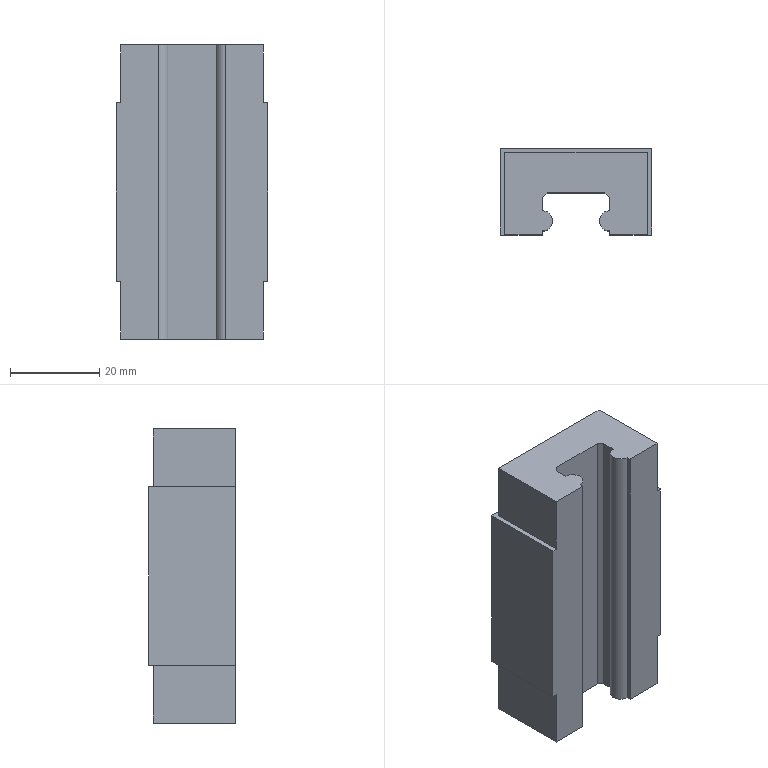Part | Creo | features CURVE 3, DATUM PLANE 3, PROTRUSION 2, COORDINATE SYSTEM 1, CUT 1 | 1 solid | 36 faces | box 34 x 19.4 x 66 mm | volume 33141 mm3 | plane 26 | cylinder 10 | commonest cylinder face diameters 3.3 x8 4.48 x2
STEP:
#1=CARTESIAN_POINT('',(0.,0.,0.));
#2=DIRECTION('',(0.,0.,1.));
#3=DIRECTION('',(1.,0.,0.));
#4=AXIS2_PLACEMENT_3D('',#1,#2,#3);
#5=CARTESIAN_POINT('',(16.,18.4,-20.));
#6=VERTEX_POINT('',#5);
#7=CARTESIAN_POINT('',(-16.,18.4,-20.));
#8=VERTEX_POINT('',#7);
#9=CARTESIAN_POINT('',(16.,18.4,-20.));
#10=DIRECTION('',(-1.,0.,0.));
#11=VECTOR('',#10,32.);
#12=LINE('',#9,#11);
#13=EDGE_CURVE('',#6,#8,#12,.T.);
#14=ORIENTED_EDGE('',*,*,#13,.F.);
#15=CARTESIAN_POINT('',(16.,0.,-20.));
#16=VERTEX_POINT('',#15);
#17=CARTESIAN_POINT('',(16.,0.,-20.));
#18=DIRECTION('',(0.,1.,0.));
#19=VECTOR('',#18,18.4);
#20=LINE('',#17,#19);
#21=EDGE_CURVE('',#16,#6,#20,.T.);
#22=ORIENTED_EDGE('',*,*,#21,.F.);
#23=CARTESIAN_POINT('',(17.,0.,-20.));
#24=VERTEX_POINT('',#23);
#25=CARTESIAN_POINT('',(16.,0.,-20.));
#26=DIRECTION('',(1.,0.,0.));
#27=VECTOR('',#26,1.);
#28=LINE('',#25,#27);
#29=EDGE_CURVE('',#16,#24,#28,.T.);
#30=ORIENTED_EDGE('',*,*,#29,.T.);
#31=CARTESIAN_POINT('',(17.,19.4,-20.));
#32=VERTEX_POINT('',#31);
#33=CARTESIAN_POINT('',(17.,0.,-20.));
#34=DIRECTION('',(0.,1.,0.));
#35=VECTOR('',#34,19.4);
#36=LINE('',#33,#35);
#37=EDGE_CURVE('',#24,#32,#36,.T.);
#38=ORIENTED_EDGE('',*,*,#37,.T.);
#39=CARTESIAN_POINT('',(-17.,19.4,-20.));
#40=VERTEX_POINT('',#39);
#41=CARTESIAN_POINT('',(17.,19.4,-20.));
#42=DIRECTION('',(-1.,0.,0.));
#43=VECTOR('',#42,34.);
#44=LINE('',#41,#43);
#45=EDGE_CURVE('',#32,#40,#44,.T.);
#46=ORIENTED_EDGE('',*,*,#45,.T.);
#47=CARTESIAN_POINT('',(-17.,0.,-20.));
#48=VERTEX_POINT('',#47);
#49=CARTESIAN_POINT('',(-17.,19.4,-20.));
#50=DIRECTION('',(0.,-1.,0.));
#51=VECTOR('',#50,19.4);
#52=LINE('',#49,#51);
#53=EDGE_CURVE('',#40,#48,#52,.T.);
#54=ORIENTED_EDGE('',*,*,#53,.T.);
#55=CARTESIAN_POINT('',(-16.,0.,-20.));
#56=VERTEX_POINT('',#55);
#57=CARTESIAN_POINT('',(-17.,0.,-20.));
#58=DIRECTION('',(1.,0.,0.));
#59=VECTOR('',#58,1.);
#60=LINE('',#57,#59);
#61=EDGE_CURVE('',#48,#56,#60,.T.);
#62=ORIENTED_EDGE('',*,*,#61,.T.);
#63=CARTESIAN_POINT('',(-16.,0.,-20.));
#64=DIRECTION('',(0.,1.,0.));
#65=VECTOR('',#64,18.4);
#66=LINE('',#63,#65);
#67=EDGE_CURVE('',#56,#8,#66,.T.);
#68=ORIENTED_EDGE('',*,*,#67,.T.);
#69=EDGE_LOOP('',(#14,#22,#30,#38,#46,#54,#62,#68));
#70=FACE_OUTER_BOUND('',#69,.F.);
#71=CARTESIAN_POINT('',(0.,0.,-20.));
#72=DIRECTION('',(0.,0.,1.));
#73=DIRECTION('',(1.,0.,0.));
#74=AXIS2_PLACEMENT_3D('',#71,#72,#73);
#75=PLANE('',#74);
#76=ADVANCED_FACE('',(#70),#75,.F.);
#77=ORIENTED_EDGE('',*,*,#13,.T.);
#78=CARTESIAN_POINT('',(-16.,18.4,-33.));
#79=VERTEX_POINT('',#78);
#80=CARTESIAN_POINT('',(-16.,18.4,-33.));
#81=DIRECTION('',(0.,0.,1.));
#82=VECTOR('',#81,13.);
#83=LINE('',#80,#82);
#84=EDGE_CURVE('',#79,#8,#83,.T.);
#85=ORIENTED_EDGE('',*,*,#84,.F.);
#86=CARTESIAN_POINT('',(16.,18.4,-33.));
#87=VERTEX_POINT('',#86);
#88=CARTESIAN_POINT('',(16.,18.4,-33.));
#89=DIRECTION('',(-1.,0.,0.));
#90=VECTOR('',#89,32.);
#91=LINE('',#88,#90);
#92=EDGE_CURVE('',#87,#79,#91,.T.);
#93=ORIENTED_EDGE('',*,*,#92,.F.);
#94=CARTESIAN_POINT('',(16.,18.4,-33.));
#95=DIRECTION('',(0.,0.,1.));
#96=VECTOR('',#95,13.);
#97=LINE('',#94,#96);
#98=EDGE_CURVE('',#87,#6,#97,.T.);
#99=ORIENTED_EDGE('',*,*,#98,.T.);
#100=EDGE_LOOP('',(#77,#85,#93,#99));
#101=FACE_OUTER_BOUND('',#100,.F.);
#102=CARTESIAN_POINT('',(16.,18.4,-33.));
#103=DIRECTION('',(0.,1.,0.));
#104=DIRECTION('',(-1.,0.,0.));
#105=AXIS2_PLACEMENT_3D('',#102,#103,#104);
#106=PLANE('',#105);
#107=ADVANCED_FACE('',(#101),#106,.T.);
#108=CARTESIAN_POINT('',(16.,18.4,20.));
#109=VERTEX_POINT('',#108);
#110=CARTESIAN_POINT('',(-16.,18.4,20.));
#111=VERTEX_POINT('',#110);
#112=CARTESIAN_POINT('',(16.,18.4,20.));
#113=DIRECTION('',(-1.,0.,0.));
#114=VECTOR('',#113,32.);
#115=LINE('',#112,#114);
#116=EDGE_CURVE('',#109,#111,#115,.T.);
#117=ORIENTED_EDGE('',*,*,#116,.F.);
#118=CARTESIAN_POINT('',(16.,18.4,33.));
#119=VERTEX_POINT('',#118);
#120=CARTESIAN_POINT('',(16.,18.4,20.));
#121=DIRECTION('',(0.,0.,1.));
#122=VECTOR('',#121,13.);
#123=LINE('',#120,#122);
#124=EDGE_CURVE('',#109,#119,#123,.T.);
#125=ORIENTED_EDGE('',*,*,#124,.T.);
#126=CARTESIAN_POINT('',(-16.,18.4,33.));
#127=VERTEX_POINT('',#126);
#128=CARTESIAN_POINT('',(16.,18.4,33.));
#129=DIRECTION('',(-1.,0.,0.));
#130=VECTOR('',#129,32.);
#131=LINE('',#128,#130);
#132=EDGE_CURVE('',#119,#127,#131,.T.);
#133=ORIENTED_EDGE('',*,*,#132,.T.);
#134=CARTESIAN_POINT('',(-16.,18.4,20.));
#135=DIRECTION('',(0.,0.,1.));
#136=VECTOR('',#135,13.);
#137=LINE('',#134,#136);
#138=EDGE_CURVE('',#111,#127,#137,.T.);
#139=ORIENTED_EDGE('',*,*,#138,.F.);
#140=EDGE_LOOP('',(#117,#125,#133,#139));
#141=FACE_OUTER_BOUND('',#140,.F.);
#142=CARTESIAN_POINT('',(16.,18.4,-33.));
#143=DIRECTION('',(0.,1.,0.));
#144=DIRECTION('',(-1.,0.,0.));
#145=AXIS2_PLACEMENT_3D('',#142,#143,#144);
#146=PLANE('',#145);
#147=ADVANCED_FACE('',(#141),#146,.T.);
#148=ORIENTED_EDGE('',*,*,#67,.F.);
#149=CARTESIAN_POINT('',(-16.,0.,-33.));
#150=VERTEX_POINT('',#149);
#151=CARTESIAN_POINT('',(-16.,0.,-33.));
#152=DIRECTION('',(0.,0.,1.));
#153=VECTOR('',#152,13.);
#154=LINE('',#151,#153);
#155=EDGE_CURVE('',#150,#56,#154,.T.);
#156=ORIENTED_EDGE('',*,*,#155,.F.);
#157=CARTESIAN_POINT('',(-16.,18.4,-33.));
#158=DIRECTION('',(0.,-1.,0.));
#159=VECTOR('',#158,18.4);
#160=LINE('',#157,#159);
#161=EDGE_CURVE('',#79,#150,#160,.T.);
#162=ORIENTED_EDGE('',*,*,#161,.F.);
#163=ORIENTED_EDGE('',*,*,#84,.T.);
#164=EDGE_LOOP('',(#148,#156,#162,#163));
#165=FACE_OUTER_BOUND('',#164,.F.);
#166=CARTESIAN_POINT('',(-16.,18.4,-33.));
#167=DIRECTION('',(-1.,0.,0.));
#168=DIRECTION('',(0.,-1.,0.));
#169=AXIS2_PLACEMENT_3D('',#166,#167,#168);
#170=PLANE('',#169);
#171=ADVANCED_FACE('',(#165),#170,.T.);
#172=CARTESIAN_POINT('',(-16.,0.,20.));
#173=VERTEX_POINT('',#172);
#174=CARTESIAN_POINT('',(-16.,0.,20.));
#175=DIRECTION('',(0.,1.,0.));
#176=VECTOR('',#175,18.4);
#177=LINE('',#174,#176);
#178=EDGE_CURVE('',#173,#111,#177,.T.);
#179=ORIENTED_EDGE('',*,*,#178,.T.);
#180=ORIENTED_EDGE('',*,*,#138,.T.);
#181=CARTESIAN_POINT('',(-16.,0.,33.));
#182=VERTEX_POINT('',#181);
#183=CARTESIAN_POINT('',(-16.,18.4,33.));
#184=DIRECTION('',(0.,-1.,0.));
#185=VECTOR('',#184,18.4);
#186=LINE('',#183,#185);
#187=EDGE_CURVE('',#127,#182,#186,.T.);
#188=ORIENTED_EDGE('',*,*,#187,.T.);
#189=CARTESIAN_POINT('',(-16.,0.,20.));
#190=DIRECTION('',(0.,0.,1.));
#191=VECTOR('',#190,13.);
#192=LINE('',#189,#191);
#193=EDGE_CURVE('',#173,#182,#192,.T.);
#194=ORIENTED_EDGE('',*,*,#193,.F.);
#195=EDGE_LOOP('',(#179,#180,#188,#194));
#196=FACE_OUTER_BOUND('',#195,.F.);
#197=CARTESIAN_POINT('',(-16.,18.4,-33.));
#198=DIRECTION('',(-1.,0.,0.));
#199=DIRECTION('',(0.,-1.,0.));
#200=AXIS2_PLACEMENT_3D('',#197,#198,#199);
#201=PLANE('',#200);
#202=ADVANCED_FACE('',(#196),#201,.T.);
#203=CARTESIAN_POINT('',(-17.,0.,20.));
#204=VERTEX_POINT('',#203);
#205=CARTESIAN_POINT('',(-17.,0.,20.));
#206=DIRECTION('',(1.,0.,0.));
#207=VECTOR('',#206,1.);
#208=LINE('',#205,#207);
#209=EDGE_CURVE('',#204,#173,#208,.T.);
#210=ORIENTED_EDGE('',*,*,#209,.T.);
#211=ORIENTED_EDGE('',*,*,#193,.T.);
#212=CARTESIAN_POINT('',(-7.5,0.,33.));
#213=VERTEX_POINT('',#212);
#214=CARTESIAN_POINT('',(-16.,0.,33.));
#215=DIRECTION('',(1.,0.,0.));
#216=VECTOR('',#215,8.5);
#217=LINE('',#214,#216);
#218=EDGE_CURVE('',#182,#213,#217,.T.);
#219=ORIENTED_EDGE('',*,*,#218,.T.);
#220=CARTESIAN_POINT('',(-7.5,0.,-33.));
#221=VERTEX_POINT('',#220);
#222=CARTESIAN_POINT('',(-7.5,0.,-33.));
#223=DIRECTION('',(0.,0.,1.));
#224=VECTOR('',#223,66.);
#225=LINE('',#222,#224);
#226=EDGE_CURVE('',#221,#213,#225,.T.);
#227=ORIENTED_EDGE('',*,*,#226,.F.);
#228=CARTESIAN_POINT('',(-16.,0.,-33.));
#229=DIRECTION('',(1.,0.,0.));
#230=VECTOR('',#229,8.5);
#231=LINE('',#228,#230);
#232=EDGE_CURVE('',#150,#221,#231,.T.);
#233=ORIENTED_EDGE('',*,*,#232,.F.);
#234=ORIENTED_EDGE('',*,*,#155,.T.);
#235=ORIENTED_EDGE('',*,*,#61,.F.);
#236=CARTESIAN_POINT('',(-17.,0.,-20.));
#237=DIRECTION('',(0.,0.,1.));
#238=VECTOR('',#237,40.);
#239=LINE('',#236,#238);
#240=EDGE_CURVE('',#48,#204,#239,.T.);
#241=ORIENTED_EDGE('',*,*,#240,.T.);
#242=EDGE_LOOP('',(#210,#211,#219,#227,#233,#234,#235,#241));
#243=FACE_OUTER_BOUND('',#242,.F.);
#244=CARTESIAN_POINT('',(-17.,0.,-20.));
#245=DIRECTION('',(0.,-1.,0.));
#246=DIRECTION('',(1.,0.,0.));
#247=AXIS2_PLACEMENT_3D('',#244,#245,#246);
#248=PLANE('',#247);
#249=ADVANCED_FACE('',(#243),#248,.T.);
#250=ORIENTED_EDGE('',*,*,#116,.T.);
#251=ORIENTED_EDGE('',*,*,#178,.F.);
#252=ORIENTED_EDGE('',*,*,#209,.F.);
#253=CARTESIAN_POINT('',(-17.,19.4,20.));
#254=VERTEX_POINT('',#253);
#255=CARTESIAN_POINT('',(-17.,19.4,20.));
#256=DIRECTION('',(0.,-1.,0.));
#257=VECTOR('',#256,19.4);
#258=LINE('',#255,#257);
#259=EDGE_CURVE('',#254,#204,#258,.T.);
#260=ORIENTED_EDGE('',*,*,#259,.F.);
#261=CARTESIAN_POINT('',(17.,19.4,20.));
#262=VERTEX_POINT('',#261);
#263=CARTESIAN_POINT('',(17.,19.4,20.));
#264=DIRECTION('',(-1.,0.,0.));
#265=VECTOR('',#264,34.);
#266=LINE('',#263,#265);
#267=EDGE_CURVE('',#262,#254,#266,.T.);
#268=ORIENTED_EDGE('',*,*,#267,.F.);
#269=CARTESIAN_POINT('',(17.,0.,20.));
#270=VERTEX_POINT('',#269);
#271=CARTESIAN_POINT('',(17.,0.,20.));
#272=DIRECTION('',(0.,1.,0.));
#273=VECTOR('',#272,19.4);
#274=LINE('',#271,#273);
#275=EDGE_CURVE('',#270,#262,#274,.T.);
#276=ORIENTED_EDGE('',*,*,#275,.F.);
#277=CARTESIAN_POINT('',(16.,0.,20.));
#278=VERTEX_POINT('',#277);
#279=CARTESIAN_POINT('',(16.,0.,20.));
#280=DIRECTION('',(1.,0.,0.));
#281=VECTOR('',#280,1.);
#282=LINE('',#279,#281);
#283=EDGE_CURVE('',#278,#270,#282,.T.);
#284=ORIENTED_EDGE('',*,*,#283,.F.);
#285=CARTESIAN_POINT('',(16.,0.,20.));
#286=DIRECTION('',(0.,1.,0.));
#287=VECTOR('',#286,18.4);
#288=LINE('',#285,#287);
#289=EDGE_CURVE('',#278,#109,#288,.T.);
#290=ORIENTED_EDGE('',*,*,#289,.T.);
#291=EDGE_LOOP('',(#250,#251,#252,#260,#268,#276,#284,#290));
#292=FACE_OUTER_BOUND('',#291,.F.);
#293=CARTESIAN_POINT('',(0.,0.,20.));
#294=DIRECTION('',(0.,0.,1.));
#295=DIRECTION('',(1.,0.,0.));
#296=AXIS2_PLACEMENT_3D('',#293,#294,#295);
#297=PLANE('',#296);
#298=ADVANCED_FACE('',(#292),#297,.T.);
#299=ORIENTED_EDGE('',*,*,#53,.F.);
#300=CARTESIAN_POINT('',(-17.,19.4,-20.));
#301=DIRECTION('',(0.,0.,1.));
#302=VECTOR('',#301,40.);
#303=LINE('',#300,#302);
#304=EDGE_CURVE('',#40,#254,#303,.T.);
#305=ORIENTED_EDGE('',*,*,#304,.T.);
#306=ORIENTED_EDGE('',*,*,#259,.T.);
#307=ORIENTED_EDGE('',*,*,#240,.F.);
#308=EDGE_LOOP('',(#299,#305,#306,#307));
#309=FACE_OUTER_BOUND('',#308,.F.);
#310=CARTESIAN_POINT('',(-17.,19.4,-20.));
#311=DIRECTION('',(-1.,0.,0.));
#312=DIRECTION('',(0.,-1.,0.));
#313=AXIS2_PLACEMENT_3D('',#310,#311,#312);
#314=PLANE('',#313);
#315=ADVANCED_FACE('',(#309),#314,.T.);
#316=ORIENTED_EDGE('',*,*,#45,.F.);
#317=CARTESIAN_POINT('',(17.,19.4,-20.));
#318=DIRECTION('',(0.,0.,1.));
#319=VECTOR('',#318,40.);
#320=LINE('',#317,#319);
#321=EDGE_CURVE('',#32,#262,#320,.T.);
#322=ORIENTED_EDGE('',*,*,#321,.T.);
#323=ORIENTED_EDGE('',*,*,#267,.T.);
#324=ORIENTED_EDGE('',*,*,#304,.F.);
#325=EDGE_LOOP('',(#316,#322,#323,#324));
#326=FACE_OUTER_BOUND('',#325,.F.);
#327=CARTESIAN_POINT('',(-11.35,19.4,-13.));
#328=VERTEX_POINT('',#327);
#329=CARTESIAN_POINT('',(-14.65,19.4,-13.));
#330=VERTEX_POINT('',#329);
#331=CARTESIAN_POINT('',(-13.,19.4,-13.));
#332=DIRECTION('',(0.,1.,0.));
#333=DIRECTION('',(1.,0.,0.));
#334=AXIS2_PLACEMENT_3D('',#331,#332,#333);
#335=CIRCLE('',#334,1.65);
#336=EDGE_CURVE('',#328,#330,#335,.T.);
#337=ORIENTED_EDGE('',*,*,#336,.T.);
#338=CARTESIAN_POINT('',(-13.,19.4,-13.));
#339=DIRECTION('',(0.,1.,0.));
#340=DIRECTION('',(-1.,0.,0.));
#341=AXIS2_PLACEMENT_3D('',#338,#339,#340);
#342=CIRCLE('',#341,1.65);
#343=EDGE_CURVE('',#330,#328,#342,.T.);
#344=ORIENTED_EDGE('',*,*,#343,.T.);
#345=EDGE_LOOP('',(#337,#344));
#346=FACE_BOUND('',#345,.F.);
#347=CARTESIAN_POINT('',(14.65,19.4,-13.));
#348=VERTEX_POINT('',#347);
#349=CARTESIAN_POINT('',(11.35,19.4,-13.));
#350=VERTEX_POINT('',#349);
#351=CARTESIAN_POINT('',(13.,19.4,-13.));
#352=DIRECTION('',(0.,1.,0.));
#353=DIRECTION('',(1.,0.,0.));
#354=AXIS2_PLACEMENT_3D('',#351,#352,#353);
#355=CIRCLE('',#354,1.65);
#356=EDGE_CURVE('',#348,#350,#355,.T.);
#357=ORIENTED_EDGE('',*,*,#356,.T.);
#358=CARTESIAN_POINT('',(13.,19.4,-13.));
#359=DIRECTION('',(0.,1.,0.));
#360=DIRECTION('',(-1.,0.,0.));
#361=AXIS2_PLACEMENT_3D('',#358,#359,#360);
#362=CIRCLE('',#361,1.65);
#363=EDGE_CURVE('',#350,#348,#362,.T.);
#364=ORIENTED_EDGE('',*,*,#363,.T.);
#365=EDGE_LOOP('',(#357,#364));
#366=FACE_BOUND('',#365,.F.);
#367=CARTESIAN_POINT('',(-11.35,19.4,13.));
#368=VERTEX_POINT('',#367);
#369=CARTESIAN_POINT('',(-14.65,19.4,13.));
#370=VERTEX_POINT('',#369);
#371=CARTESIAN_POINT('',(-13.,19.4,13.));
#372=DIRECTION('',(0.,1.,0.));
#373=DIRECTION('',(1.,0.,0.));
#374=AXIS2_PLACEMENT_3D('',#371,#372,#373);
#375=CIRCLE('',#374,1.65);
#376=EDGE_CURVE('',#368,#370,#375,.T.);
#377=ORIENTED_EDGE('',*,*,#376,.T.);
#378=CARTESIAN_POINT('',(-13.,19.4,13.));
#379=DIRECTION('',(0.,1.,0.));
#380=DIRECTION('',(-1.,0.,0.));
#381=AXIS2_PLACEMENT_3D('',#378,#379,#380);
#382=CIRCLE('',#381,1.65);
#383=EDGE_CURVE('',#370,#368,#382,.T.);
#384=ORIENTED_EDGE('',*,*,#383,.T.);
#385=EDGE_LOOP('',(#377,#384));
#386=FACE_BOUND('',#385,.F.);
#387=CARTESIAN_POINT('',(14.65,19.4,13.));
#388=VERTEX_POINT('',#387);
#389=CARTESIAN_POINT('',(11.35,19.4,13.));
#390=VERTEX_POINT('',#389);
#391=CARTESIAN_POINT('',(13.,19.4,13.));
#392=DIRECTION('',(0.,1.,0.));
#393=DIRECTION('',(1.,0.,0.));
#394=AXIS2_PLACEMENT_3D('',#391,#392,#393);
#395=CIRCLE('',#394,1.65);
#396=EDGE_CURVE('',#388,#390,#395,.T.);
#397=ORIENTED_EDGE('',*,*,#396,.T.);
#398=CARTESIAN_POINT('',(13.,19.4,13.));
#399=DIRECTION('',(0.,1.,0.));
#400=DIRECTION('',(-1.,0.,0.));
#401=AXIS2_PLACEMENT_3D('',#398,#399,#400);
#402=CIRCLE('',#401,1.65);
#403=EDGE_CURVE('',#390,#388,#402,.T.);
#404=ORIENTED_EDGE('',*,*,#403,.T.);
#405=EDGE_LOOP('',(#397,#404));
#406=FACE_BOUND('',#405,.F.);
#407=CARTESIAN_POINT('',(17.,19.4,-20.));
#408=DIRECTION('',(0.,1.,0.));
#409=DIRECTION('',(-1.,0.,0.));
#410=AXIS2_PLACEMENT_3D('',#407,#408,#409);
#411=PLANE('',#410);
#412=ADVANCED_FACE('',(#326,#346,#366,#386,#406),#411,.T.);
#413=ORIENTED_EDGE('',*,*,#37,.F.);
#414=CARTESIAN_POINT('',(17.,0.,-20.));
#415=DIRECTION('',(0.,0.,1.));
#416=VECTOR('',#415,40.);
#417=LINE('',#414,#416);
#418=EDGE_CURVE('',#24,#270,#417,.T.);
#419=ORIENTED_EDGE('',*,*,#418,.T.);
#420=ORIENTED_EDGE('',*,*,#275,.T.);
#421=ORIENTED_EDGE('',*,*,#321,.F.);
#422=EDGE_LOOP('',(#413,#419,#420,#421));
#423=FACE_OUTER_BOUND('',#422,.F.);
#424=CARTESIAN_POINT('',(17.,0.,-20.));
#425=DIRECTION('',(1.,0.,0.));
#426=DIRECTION('',(0.,1.,0.));
#427=AXIS2_PLACEMENT_3D('',#424,#425,#426);
#428=PLANE('',#427);
#429=ADVANCED_FACE('',(#423),#428,.T.);
#430=CARTESIAN_POINT('',(7.5,0.,-33.));
#431=VERTEX_POINT('',#430);
#432=CARTESIAN_POINT('',(7.5,0.,33.));
#433=VERTEX_POINT('',#432);
#434=CARTESIAN_POINT('',(7.5,0.,-33.));
#435=DIRECTION('',(0.,0.,1.));
#436=VECTOR('',#435,66.);
#437=LINE('',#434,#436);
#438=EDGE_CURVE('',#431,#433,#437,.T.);
#439=ORIENTED_EDGE('',*,*,#438,.T.);
#440=CARTESIAN_POINT('',(16.,0.,33.));
#441=VERTEX_POINT('',#440);
#442=CARTESIAN_POINT('',(7.5,0.,33.));
#443=DIRECTION('',(1.,0.,0.));
#444=VECTOR('',#443,8.5);
#445=LINE('',#442,#444);
#446=EDGE_CURVE('',#433,#441,#445,.T.);
#447=ORIENTED_EDGE('',*,*,#446,.T.);
#448=CARTESIAN_POINT('',(16.,0.,20.));
#449=DIRECTION('',(0.,0.,1.));
#450=VECTOR('',#449,13.);
#451=LINE('',#448,#450);
#452=EDGE_CURVE('',#278,#441,#451,.T.);
#453=ORIENTED_EDGE('',*,*,#452,.F.);
#454=ORIENTED_EDGE('',*,*,#283,.T.);
#455=ORIENTED_EDGE('',*,*,#418,.F.);
#456=ORIENTED_EDGE('',*,*,#29,.F.);
#457=CARTESIAN_POINT('',(16.,0.,-33.));
#458=VERTEX_POINT('',#457);
#459=CARTESIAN_POINT('',(16.,0.,-33.));
#460=DIRECTION('',(0.,0.,1.));
#461=VECTOR('',#460,13.);
#462=LINE('',#459,#461);
#463=EDGE_CURVE('',#458,#16,#462,.T.);
#464=ORIENTED_EDGE('',*,*,#463,.F.);
#465=CARTESIAN_POINT('',(7.5,0.,-33.));
#466=DIRECTION('',(1.,0.,0.));
#467=VECTOR('',#466,8.5);
#468=LINE('',#465,#467);
#469=EDGE_CURVE('',#431,#458,#468,.T.);
#470=ORIENTED_EDGE('',*,*,#469,.F.);
#471=EDGE_LOOP('',(#439,#447,#453,#454,#455,#456,#464,#470));
#472=FACE_OUTER_BOUND('',#471,.F.);
#473=CARTESIAN_POINT('',(7.5,0.,-20.));
#474=DIRECTION('',(0.,-1.,0.));
#475=DIRECTION('',(1.,0.,0.));
#476=AXIS2_PLACEMENT_3D('',#473,#474,#475);
#477=PLANE('',#476);
#478=ADVANCED_FACE('',(#472),#477,.T.);
#479=CARTESIAN_POINT('',(7.5,0.93,-33.));
#480=VERTEX_POINT('',#479);
#481=CARTESIAN_POINT('',(7.5,0.93,33.));
#482=VERTEX_POINT('',#481);
#483=CARTESIAN_POINT('',(7.5,0.93,-33.));
#484=DIRECTION('',(0.,0.,1.));
#485=VECTOR('',#484,66.);
#486=LINE('',#483,#485);
#487=EDGE_CURVE('',#480,#482,#486,.T.);
#488=ORIENTED_EDGE('',*,*,#487,.T.);
#489=CARTESIAN_POINT('',(7.5,0.93,33.));
#490=DIRECTION('',(0.,-1.,0.));
#491=VECTOR('',#490,0.93);
#492=LINE('',#489,#491);
#493=EDGE_CURVE('',#482,#433,#492,.T.);
#494=ORIENTED_EDGE('',*,*,#493,.T.);
#495=ORIENTED_EDGE('',*,*,#438,.F.);
#496=CARTESIAN_POINT('',(7.5,0.93,-33.));
#497=DIRECTION('',(0.,-1.,0.));
#498=VECTOR('',#497,0.93);
#499=LINE('',#496,#498);
#500=EDGE_CURVE('',#480,#431,#499,.T.);
#501=ORIENTED_EDGE('',*,*,#500,.F.);
#502=EDGE_LOOP('',(#488,#494,#495,#501));
#503=FACE_OUTER_BOUND('',#502,.F.);
#504=CARTESIAN_POINT('',(7.5,0.93,-20.));
#505=DIRECTION('',(-1.,0.,0.));
#506=DIRECTION('',(0.,-1.,0.));
#507=AXIS2_PLACEMENT_3D('',#504,#505,#506);
#508=PLANE('',#507);
#509=ADVANCED_FACE('',(#503),#508,.T.);
#510=CARTESIAN_POINT('',(7.5,5.41,-33.));
#511=VERTEX_POINT('',#510);
#512=CARTESIAN_POINT('',(7.5,5.41,33.));
#513=VERTEX_POINT('',#512);
#514=CARTESIAN_POINT('',(7.5,5.41,-33.));
#515=DIRECTION('',(0.,0.,1.));
#516=VECTOR('',#515,66.);
#517=LINE('',#514,#516);
#518=EDGE_CURVE('',#511,#513,#517,.T.);
#519=ORIENTED_EDGE('',*,*,#518,.T.);
#520=CARTESIAN_POINT('',(7.5,3.17,33.));
#521=DIRECTION('',(0.,0.,1.));
#522=DIRECTION('',(0.,1.,0.));
#523=AXIS2_PLACEMENT_3D('',#520,#521,#522);
#524=CIRCLE('',#523,2.24);
#525=EDGE_CURVE('',#513,#482,#524,.T.);
#526=ORIENTED_EDGE('',*,*,#525,.T.);
#527=ORIENTED_EDGE('',*,*,#487,.F.);
#528=CARTESIAN_POINT('',(7.5,3.17,-33.));
#529=DIRECTION('',(0.,0.,1.));
#530=DIRECTION('',(0.,1.,0.));
#531=AXIS2_PLACEMENT_3D('',#528,#529,#530);
#532=CIRCLE('',#531,2.24);
#533=EDGE_CURVE('',#511,#480,#532,.T.);
#534=ORIENTED_EDGE('',*,*,#533,.F.);
#535=EDGE_LOOP('',(#519,#526,#527,#534));
#536=FACE_OUTER_BOUND('',#535,.F.);
#537=CARTESIAN_POINT('',(7.5,3.17,-20.));
#538=DIRECTION('',(0.,0.,1.));
#539=DIRECTION('',(1.,0.,0.));
#540=AXIS2_PLACEMENT_3D('',#537,#538,#539);
#541=CYLINDRICAL_SURFACE('',#540,2.24);
#542=ADVANCED_FACE('',(#536),#541,.T.);
#543=CARTESIAN_POINT('',(7.5,8.41,-33.));
#544=VERTEX_POINT('',#543);
#545=CARTESIAN_POINT('',(7.5,8.41,33.));
#546=VERTEX_POINT('',#545);
#547=CARTESIAN_POINT('',(7.5,8.41,-33.));
#548=DIRECTION('',(0.,0.,1.));
#549=VECTOR('',#548,66.);
#550=LINE('',#547,#549);
#551=EDGE_CURVE('',#544,#546,#550,.T.);
#552=ORIENTED_EDGE('',*,*,#551,.T.);
#553=CARTESIAN_POINT('',(7.5,8.41,33.));
#554=DIRECTION('',(0.,-1.,0.));
#555=VECTOR('',#554,3.);
#556=LINE('',#553,#555);
#557=EDGE_CURVE('',#546,#513,#556,.T.);
#558=ORIENTED_EDGE('',*,*,#557,.T.);
#559=ORIENTED_EDGE('',*,*,#518,.F.);
#560=CARTESIAN_POINT('',(7.5,8.41,-33.));
#561=DIRECTION('',(0.,-1.,0.));
#562=VECTOR('',#561,3.);
#563=LINE('',#560,#562);
#564=EDGE_CURVE('',#544,#511,#563,.T.);
#565=ORIENTED_EDGE('',*,*,#564,.F.);
#566=EDGE_LOOP('',(#552,#558,#559,#565));
#567=FACE_OUTER_BOUND('',#566,.F.);
#568=CARTESIAN_POINT('',(7.5,8.41,-20.));
#569=DIRECTION('',(-1.,0.,0.));
#570=DIRECTION('',(0.,-1.,0.));
#571=AXIS2_PLACEMENT_3D('',#568,#569,#570);
#572=PLANE('',#571);
#573=ADVANCED_FACE('',(#567),#572,.T.);
#574=CARTESIAN_POINT('',(6.5,9.41,-33.));
#575=VERTEX_POINT('',#574);
#576=CARTESIAN_POINT('',(6.5,9.41,33.));
#577=VERTEX_POINT('',#576);
#578=CARTESIAN_POINT('',(6.5,9.41,-33.));
#579=DIRECTION('',(0.,0.,1.));
#580=VECTOR('',#579,66.);
#581=LINE('',#578,#580);
#582=EDGE_CURVE('',#575,#577,#581,.T.);
#583=ORIENTED_EDGE('',*,*,#582,.T.);
#584=CARTESIAN_POINT('',(6.5,9.41,33.));
#585=DIRECTION('',(0.7071,-0.7071,0.));
#586=VECTOR('',#585,1.414);
#587=LINE('',#584,#586);
#588=EDGE_CURVE('',#577,#546,#587,.T.);
#589=ORIENTED_EDGE('',*,*,#588,.T.);
#590=ORIENTED_EDGE('',*,*,#551,.F.);
#591=CARTESIAN_POINT('',(6.5,9.41,-33.));
#592=DIRECTION('',(0.7071,-0.7071,0.));
#593=VECTOR('',#592,1.414);
#594=LINE('',#591,#593);
#595=EDGE_CURVE('',#575,#544,#594,.T.);
#596=ORIENTED_EDGE('',*,*,#595,.F.);
#597=EDGE_LOOP('',(#583,#589,#590,#596));
#598=FACE_OUTER_BOUND('',#597,.F.);
#599=CARTESIAN_POINT('',(6.5,9.41,-20.));
#600=DIRECTION('',(-0.7071,-0.7071,0.));
#601=DIRECTION('',(0.7071,-0.7071,0.));
#602=AXIS2_PLACEMENT_3D('',#599,#600,#601);
#603=PLANE('',#602);
#604=ADVANCED_FACE('',(#598),#603,.T.);
#605=CARTESIAN_POINT('',(-6.5,9.41,-33.));
#606=VERTEX_POINT('',#605);
#607=CARTESIAN_POINT('',(-6.5,9.41,33.));
#608=VERTEX_POINT('',#607);
#609=CARTESIAN_POINT('',(-6.5,9.41,-33.));
#610=DIRECTION('',(0.,0.,1.));
#611=VECTOR('',#610,66.);
#612=LINE('',#609,#611);
#613=EDGE_CURVE('',#606,#608,#612,.T.);
#614=ORIENTED_EDGE('',*,*,#613,.T.);
#615=CARTESIAN_POINT('',(-6.5,9.41,33.));
#616=DIRECTION('',(1.,0.,0.));
#617=VECTOR('',#616,13.);
#618=LINE('',#615,#617);
#619=EDGE_CURVE('',#608,#577,#618,.T.);
#620=ORIENTED_EDGE('',*,*,#619,.T.);
#621=ORIENTED_EDGE('',*,*,#582,.F.);
#622=CARTESIAN_POINT('',(-6.5,9.41,-33.));
#623=DIRECTION('',(1.,0.,0.));
#624=VECTOR('',#623,13.);
#625=LINE('',#622,#624);
#626=EDGE_CURVE('',#606,#575,#625,.T.);
#627=ORIENTED_EDGE('',*,*,#626,.F.);
#628=EDGE_LOOP('',(#614,#620,#621,#627));
#629=FACE_OUTER_BOUND('',#628,.F.);
#630=CARTESIAN_POINT('',(-6.5,9.41,-20.));
#631=DIRECTION('',(0.,-1.,0.));
#632=DIRECTION('',(1.,0.,0.));
#633=AXIS2_PLACEMENT_3D('',#630,#631,#632);
#634=PLANE('',#633);
#635=ADVANCED_FACE('',(#629),#634,.T.);
#636=CARTESIAN_POINT('',(-7.5,8.41,-33.));
#637=VERTEX_POINT('',#636);
#638=CARTESIAN_POINT('',(-7.5,8.41,33.));
#639=VERTEX_POINT('',#638);
#640=CARTESIAN_POINT('',(-7.5,8.41,-33.));
#641=DIRECTION('',(0.,0.,1.));
#642=VECTOR('',#641,66.);
#643=LINE('',#640,#642);
#644=EDGE_CURVE('',#637,#639,#643,.T.);
#645=ORIENTED_EDGE('',*,*,#644,.T.);
#646=CARTESIAN_POINT('',(-7.5,8.41,33.));
#647=DIRECTION('',(0.7071,0.7071,0.));
#648=VECTOR('',#647,1.414);
#649=LINE('',#646,#648);
#650=EDGE_CURVE('',#639,#608,#649,.T.);
#651=ORIENTED_EDGE('',*,*,#650,.T.);
#652=ORIENTED_EDGE('',*,*,#613,.F.);
#653=CARTESIAN_POINT('',(-7.5,8.41,-33.));
#654=DIRECTION('',(0.7071,0.7071,0.));
#655=VECTOR('',#654,1.414);
#656=LINE('',#653,#655);
#657=EDGE_CURVE('',#637,#606,#656,.T.);
#658=ORIENTED_EDGE('',*,*,#657,.F.);
#659=EDGE_LOOP('',(#645,#651,#652,#658));
#660=FACE_OUTER_BOUND('',#659,.F.);
#661=CARTESIAN_POINT('',(-7.5,8.41,-20.));
#662=DIRECTION('',(0.7071,-0.7071,0.));
#663=DIRECTION('',(0.7071,0.7071,0.));
#664=AXIS2_PLACEMENT_3D('',#661,#662,#663);
#665=PLANE('',#664);
#666=ADVANCED_FACE('',(#660),#665,.T.);
#667=CARTESIAN_POINT('',(-7.5,5.41,-33.));
#668=VERTEX_POINT('',#667);
#669=CARTESIAN_POINT('',(-7.5,5.41,33.));
#670=VERTEX_POINT('',#669);
#671=CARTESIAN_POINT('',(-7.5,5.41,-33.));
#672=DIRECTION('',(0.,0.,1.));
#673=VECTOR('',#672,66.);
#674=LINE('',#671,#673);
#675=EDGE_CURVE('',#668,#670,#674,.T.);
#676=ORIENTED_EDGE('',*,*,#675,.T.);
#677=CARTESIAN_POINT('',(-7.5,5.41,33.));
#678=DIRECTION('',(0.,1.,0.));
#679=VECTOR('',#678,3.);
#680=LINE('',#677,#679);
#681=EDGE_CURVE('',#670,#639,#680,.T.);
#682=ORIENTED_EDGE('',*,*,#681,.T.);
#683=ORIENTED_EDGE('',*,*,#644,.F.);
#684=CARTESIAN_POINT('',(-7.5,5.41,-33.));
#685=DIRECTION('',(0.,1.,0.));
#686=VECTOR('',#685,3.);
#687=LINE('',#684,#686);
#688=EDGE_CURVE('',#668,#637,#687,.T.);
#689=ORIENTED_EDGE('',*,*,#688,.F.);
#690=EDGE_LOOP('',(#676,#682,#683,#689));
#691=FACE_OUTER_BOUND('',#690,.F.);
#692=CARTESIAN_POINT('',(-7.5,5.41,-20.));
#693=DIRECTION('',(1.,0.,0.));
#694=DIRECTION('',(0.,1.,0.));
#695=AXIS2_PLACEMENT_3D('',#692,#693,#694);
#696=PLANE('',#695);
#697=ADVANCED_FACE('',(#691),#696,.T.);
#698=CARTESIAN_POINT('',(-7.5,0.93,-33.));
#699=VERTEX_POINT('',#698);
#700=CARTESIAN_POINT('',(-7.5,0.93,33.));
#701=VERTEX_POINT('',#700);
#702=CARTESIAN_POINT('',(-7.5,0.93,-33.));
#703=DIRECTION('',(0.,0.,1.));
#704=VECTOR('',#703,66.);
#705=LINE('',#702,#704);
#706=EDGE_CURVE('',#699,#701,#705,.T.);
#707=ORIENTED_EDGE('',*,*,#706,.T.);
#708=CARTESIAN_POINT('',(-7.5,3.17,33.));
#709=DIRECTION('',(0.,0.,1.));
#710=DIRECTION('',(0.,-1.,0.));
#711=AXIS2_PLACEMENT_3D('',#708,#709,#710);
#712=CIRCLE('',#711,2.24);
#713=EDGE_CURVE('',#701,#670,#712,.T.);
#714=ORIENTED_EDGE('',*,*,#713,.T.);
#715=ORIENTED_EDGE('',*,*,#675,.F.);
#716=CARTESIAN_POINT('',(-7.5,3.17,-33.));
#717=DIRECTION('',(0.,0.,1.));
#718=DIRECTION('',(0.,-1.,0.));
#719=AXIS2_PLACEMENT_3D('',#716,#717,#718);
#720=CIRCLE('',#719,2.24);
#721=EDGE_CURVE('',#699,#668,#720,.T.);
#722=ORIENTED_EDGE('',*,*,#721,.F.);
#723=EDGE_LOOP('',(#707,#714,#715,#722));
#724=FACE_OUTER_BOUND('',#723,.F.);
#725=CARTESIAN_POINT('',(-7.5,3.17,-20.));
#726=DIRECTION('',(0.,0.,1.));
#727=DIRECTION('',(1.,0.,0.));
#728=AXIS2_PLACEMENT_3D('',#725,#726,#727);
#729=CYLINDRICAL_SURFACE('',#728,2.24);
#730=ADVANCED_FACE('',(#724),#729,.T.);
#731=ORIENTED_EDGE('',*,*,#226,.T.);
#732=CARTESIAN_POINT('',(-7.5,0.,33.));
#733=DIRECTION('',(0.,1.,0.));
#734=VECTOR('',#733,0.93);
#735=LINE('',#732,#734);
#736=EDGE_CURVE('',#213,#701,#735,.T.);
#737=ORIENTED_EDGE('',*,*,#736,.T.);
#738=ORIENTED_EDGE('',*,*,#706,.F.);
#739=CARTESIAN_POINT('',(-7.5,0.,-33.));
#740=DIRECTION('',(0.,1.,0.));
#741=VECTOR('',#740,0.93);
#742=LINE('',#739,#741);
#743=EDGE_CURVE('',#221,#699,#742,.T.);
#744=ORIENTED_EDGE('',*,*,#743,.F.);
#745=EDGE_LOOP('',(#731,#737,#738,#744));
#746=FACE_OUTER_BOUND('',#745,.F.);
#747=CARTESIAN_POINT('',(-7.5,0.,-20.));
#748=DIRECTION('',(1.,0.,0.));
#749=DIRECTION('',(0.,1.,0.));
#750=AXIS2_PLACEMENT_3D('',#747,#748,#749);
#751=PLANE('',#750);
#752=ADVANCED_FACE('',(#746),#751,.T.);
#753=ORIENTED_EDGE('',*,*,#132,.F.);
#754=CARTESIAN_POINT('',(16.,0.,33.));
#755=DIRECTION('',(0.,1.,0.));
#756=VECTOR('',#755,18.4);
#757=LINE('',#754,#756);
#758=EDGE_CURVE('',#441,#119,#757,.T.);
#759=ORIENTED_EDGE('',*,*,#758,.F.);
#760=ORIENTED_EDGE('',*,*,#446,.F.);
#761=ORIENTED_EDGE('',*,*,#493,.F.);
#762=ORIENTED_EDGE('',*,*,#525,.F.);
#763=ORIENTED_EDGE('',*,*,#557,.F.);
#764=ORIENTED_EDGE('',*,*,#588,.F.);
#765=ORIENTED_EDGE('',*,*,#619,.F.);
#766=ORIENTED_EDGE('',*,*,#650,.F.);
#767=ORIENTED_EDGE('',*,*,#681,.F.);
#768=ORIENTED_EDGE('',*,*,#713,.F.);
#769=ORIENTED_EDGE('',*,*,#736,.F.);
#770=ORIENTED_EDGE('',*,*,#218,.F.);
#771=ORIENTED_EDGE('',*,*,#187,.F.);
#772=EDGE_LOOP('',(#753,#759,#760,#761,#762,#763,#764,#765,#766,#767,#768,#769,#770,#771));
#773=FACE_OUTER_BOUND('',#772,.F.);
#774=CARTESIAN_POINT('',(0.,0.,33.));
#775=DIRECTION('',(0.,0.,1.));
#776=DIRECTION('',(1.,0.,0.));
#777=AXIS2_PLACEMENT_3D('',#774,#775,#776);
#778=PLANE('',#777);
#779=ADVANCED_FACE('',(#773),#778,.T.);
#780=ORIENTED_EDGE('',*,*,#21,.T.);
#781=ORIENTED_EDGE('',*,*,#98,.F.);
#782=CARTESIAN_POINT('',(16.,0.,-33.));
#783=DIRECTION('',(0.,1.,0.));
#784=VECTOR('',#783,18.4);
#785=LINE('',#782,#784);
#786=EDGE_CURVE('',#458,#87,#785,.T.);
#787=ORIENTED_EDGE('',*,*,#786,.F.);
#788=ORIENTED_EDGE('',*,*,#463,.T.);
#789=EDGE_LOOP('',(#780,#781,#787,#788));
#790=FACE_OUTER_BOUND('',#789,.F.);
#791=CARTESIAN_POINT('',(16.,0.,-33.));
#792=DIRECTION('',(1.,0.,0.));
#793=DIRECTION('',(0.,1.,0.));
#794=AXIS2_PLACEMENT_3D('',#791,#792,#793);
#795=PLANE('',#794);
#796=ADVANCED_FACE('',(#790),#795,.T.);
#797=ORIENTED_EDGE('',*,*,#289,.F.);
#798=ORIENTED_EDGE('',*,*,#452,.T.);
#799=ORIENTED_EDGE('',*,*,#758,.T.);
#800=ORIENTED_EDGE('',*,*,#124,.F.);
#801=EDGE_LOOP('',(#797,#798,#799,#800));
#802=FACE_OUTER_BOUND('',#801,.F.);
#803=CARTESIAN_POINT('',(16.,0.,-33.));
#804=DIRECTION('',(1.,0.,0.));
#805=DIRECTION('',(0.,1.,0.));
#806=AXIS2_PLACEMENT_3D('',#803,#804,#805);
#807=PLANE('',#806);
#808=ADVANCED_FACE('',(#802),#807,.T.);
#809=ORIENTED_EDGE('',*,*,#92,.T.);
#810=ORIENTED_EDGE('',*,*,#161,.T.);
#811=ORIENTED_EDGE('',*,*,#232,.T.);
#812=ORIENTED_EDGE('',*,*,#743,.T.);
#813=ORIENTED_EDGE('',*,*,#721,.T.);
#814=ORIENTED_EDGE('',*,*,#688,.T.);
#815=ORIENTED_EDGE('',*,*,#657,.T.);
#816=ORIENTED_EDGE('',*,*,#626,.T.);
#817=ORIENTED_EDGE('',*,*,#595,.T.);
#818=ORIENTED_EDGE('',*,*,#564,.T.);
#819=ORIENTED_EDGE('',*,*,#533,.T.);
#820=ORIENTED_EDGE('',*,*,#500,.T.);
#821=ORIENTED_EDGE('',*,*,#469,.T.);
#822=ORIENTED_EDGE('',*,*,#786,.T.);
#823=EDGE_LOOP('',(#809,#810,#811,#812,#813,#814,#815,#816,#817,#818,#819,#820,#821,#822));
#824=FACE_OUTER_BOUND('',#823,.F.);
#825=CARTESIAN_POINT('',(0.,0.,-33.));
#826=DIRECTION('',(0.,0.,1.));
#827=DIRECTION('',(1.,0.,0.));
#828=AXIS2_PLACEMENT_3D('',#825,#826,#827);
#829=PLANE('',#828);
#830=ADVANCED_FACE('',(#824),#829,.F.);
#831=ORIENTED_EDGE('',*,*,#336,.F.);
#832=CARTESIAN_POINT('',(-11.35,9.4,-13.));
#833=VERTEX_POINT('',#832);
#834=CARTESIAN_POINT('',(-11.35,19.4,-13.));
#835=DIRECTION('',(0.,-1.,0.));
#836=VECTOR('',#835,10.);
#837=LINE('',#834,#836);
#838=EDGE_CURVE('',#328,#833,#837,.T.);
#839=ORIENTED_EDGE('',*,*,#838,.T.);
#840=CARTESIAN_POINT('',(-14.65,9.4,-13.));
#841=VERTEX_POINT('',#840);
#842=CARTESIAN_POINT('',(-13.,9.4,-13.));
#843=DIRECTION('',(0.,1.,0.));
#844=DIRECTION('',(1.,0.,0.));
#845=AXIS2_PLACEMENT_3D('',#842,#843,#844);
#846=CIRCLE('',#845,1.65);
#847=EDGE_CURVE('',#833,#841,#846,.T.);
#848=ORIENTED_EDGE('',*,*,#847,.T.);
#849=CARTESIAN_POINT('',(-14.65,19.4,-13.));
#850=DIRECTION('',(0.,-1.,0.));
#851=VECTOR('',#850,10.);
#852=LINE('',#849,#851);
#853=EDGE_CURVE('',#330,#841,#852,.T.);
#854=ORIENTED_EDGE('',*,*,#853,.F.);
#855=EDGE_LOOP('',(#831,#839,#848,#854));
#856=FACE_OUTER_BOUND('',#855,.F.);
#857=CARTESIAN_POINT('',(-13.,19.4,-13.));
#858=DIRECTION('',(0.,1.,0.));
#859=DIRECTION('',(1.,0.,0.));
#860=AXIS2_PLACEMENT_3D('',#857,#858,#859);
#861=CYLINDRICAL_SURFACE('',#860,1.65);
#862=ADVANCED_FACE('',(#856),#861,.F.);
#863=ORIENTED_EDGE('',*,*,#343,.F.);
#864=ORIENTED_EDGE('',*,*,#853,.T.);
#865=CARTESIAN_POINT('',(-13.,9.4,-13.));
#866=DIRECTION('',(0.,1.,0.));
#867=DIRECTION('',(-1.,0.,0.));
#868=AXIS2_PLACEMENT_3D('',#865,#866,#867);
#869=CIRCLE('',#868,1.65);
#870=EDGE_CURVE('',#841,#833,#869,.T.);
#871=ORIENTED_EDGE('',*,*,#870,.T.);
#872=ORIENTED_EDGE('',*,*,#838,.F.);
#873=EDGE_LOOP('',(#863,#864,#871,#872));
#874=FACE_OUTER_BOUND('',#873,.F.);
#875=CARTESIAN_POINT('',(-13.,19.4,-13.));
#876=DIRECTION('',(0.,1.,0.));
#877=DIRECTION('',(1.,0.,0.));
#878=AXIS2_PLACEMENT_3D('',#875,#876,#877);
#879=CYLINDRICAL_SURFACE('',#878,1.65);
#880=ADVANCED_FACE('',(#874),#879,.F.);
#881=ORIENTED_EDGE('',*,*,#847,.F.);
#882=ORIENTED_EDGE('',*,*,#870,.F.);
#883=EDGE_LOOP('',(#881,#882));
#884=FACE_OUTER_BOUND('',#883,.F.);
#885=CARTESIAN_POINT('',(0.,9.4,-20.));
#886=DIRECTION('',(0.,1.,0.));
#887=DIRECTION('',(1.,0.,0.));
#888=AXIS2_PLACEMENT_3D('',#885,#886,#887);
#889=PLANE('',#888);
#890=ADVANCED_FACE('',(#884),#889,.T.);
#891=CARTESIAN_POINT('',(14.65,9.4,-13.));
#892=VERTEX_POINT('',#891);
#893=CARTESIAN_POINT('',(11.35,9.4,-13.));
#894=VERTEX_POINT('',#893);
#895=CARTESIAN_POINT('',(13.,9.4,-13.));
#896=DIRECTION('',(0.,1.,0.));
#897=DIRECTION('',(1.,0.,0.));
#898=AXIS2_PLACEMENT_3D('',#895,#896,#897);
#899=CIRCLE('',#898,1.65);
#900=EDGE_CURVE('',#892,#894,#899,.T.);
#901=ORIENTED_EDGE('',*,*,#900,.F.);
#902=CARTESIAN_POINT('',(13.,9.4,-13.));
#903=DIRECTION('',(0.,1.,0.));
#904=DIRECTION('',(-1.,0.,0.));
#905=AXIS2_PLACEMENT_3D('',#902,#903,#904);
#906=CIRCLE('',#905,1.65);
#907=EDGE_CURVE('',#894,#892,#906,.T.);
#908=ORIENTED_EDGE('',*,*,#907,.F.);
#909=EDGE_LOOP('',(#901,#908));
#910=FACE_OUTER_BOUND('',#909,.F.);
#911=CARTESIAN_POINT('',(0.,9.4,-20.));
#912=DIRECTION('',(0.,1.,0.));
#913=DIRECTION('',(1.,0.,0.));
#914=AXIS2_PLACEMENT_3D('',#911,#912,#913);
#915=PLANE('',#914);
#916=ADVANCED_FACE('',(#910),#915,.T.);
#917=CARTESIAN_POINT('',(-11.35,9.4,13.));
#918=VERTEX_POINT('',#917);
#919=CARTESIAN_POINT('',(-14.65,9.4,13.));
#920=VERTEX_POINT('',#919);
#921=CARTESIAN_POINT('',(-13.,9.4,13.));
#922=DIRECTION('',(0.,1.,0.));
#923=DIRECTION('',(1.,0.,0.));
#924=AXIS2_PLACEMENT_3D('',#921,#922,#923);
#925=CIRCLE('',#924,1.65);
#926=EDGE_CURVE('',#918,#920,#925,.T.);
#927=ORIENTED_EDGE('',*,*,#926,.F.);
#928=CARTESIAN_POINT('',(-13.,9.4,13.));
#929=DIRECTION('',(0.,1.,0.));
#930=DIRECTION('',(-1.,0.,0.));
#931=AXIS2_PLACEMENT_3D('',#928,#929,#930);
#932=CIRCLE('',#931,1.65);
#933=EDGE_CURVE('',#920,#918,#932,.T.);
#934=ORIENTED_EDGE('',*,*,#933,.F.);
#935=EDGE_LOOP('',(#927,#934));
#936=FACE_OUTER_BOUND('',#935,.F.);
#937=CARTESIAN_POINT('',(0.,9.4,-20.));
#938=DIRECTION('',(0.,1.,0.));
#939=DIRECTION('',(1.,0.,0.));
#940=AXIS2_PLACEMENT_3D('',#937,#938,#939);
#941=PLANE('',#940);
#942=ADVANCED_FACE('',(#936),#941,.T.);
#943=CARTESIAN_POINT('',(14.65,9.4,13.));
#944=VERTEX_POINT('',#943);
#945=CARTESIAN_POINT('',(11.35,9.4,13.));
#946=VERTEX_POINT('',#945);
#947=CARTESIAN_POINT('',(13.,9.4,13.));
#948=DIRECTION('',(0.,1.,0.));
#949=DIRECTION('',(1.,0.,0.));
#950=AXIS2_PLACEMENT_3D('',#947,#948,#949);
#951=CIRCLE('',#950,1.65);
#952=EDGE_CURVE('',#944,#946,#951,.T.);
#953=ORIENTED_EDGE('',*,*,#952,.F.);
#954=CARTESIAN_POINT('',(13.,9.4,13.));
#955=DIRECTION('',(0.,1.,0.));
#956=DIRECTION('',(-1.,0.,0.));
#957=AXIS2_PLACEMENT_3D('',#954,#955,#956);
#958=CIRCLE('',#957,1.65);
#959=EDGE_CURVE('',#946,#944,#958,.T.);
#960=ORIENTED_EDGE('',*,*,#959,.F.);
#961=EDGE_LOOP('',(#953,#960));
#962=FACE_OUTER_BOUND('',#961,.F.);
#963=CARTESIAN_POINT('',(0.,9.4,-20.));
#964=DIRECTION('',(0.,1.,0.));
#965=DIRECTION('',(1.,0.,0.));
#966=AXIS2_PLACEMENT_3D('',#963,#964,#965);
#967=PLANE('',#966);
#968=ADVANCED_FACE('',(#962),#967,.T.);
#969=ORIENTED_EDGE('',*,*,#356,.F.);
#970=CARTESIAN_POINT('',(14.65,19.4,-13.));
#971=DIRECTION('',(0.,-1.,0.));
#972=VECTOR('',#971,10.);
#973=LINE('',#970,#972);
#974=EDGE_CURVE('',#348,#892,#973,.T.);
#975=ORIENTED_EDGE('',*,*,#974,.T.);
#976=ORIENTED_EDGE('',*,*,#900,.T.);
#977=CARTESIAN_POINT('',(11.35,19.4,-13.));
#978=DIRECTION('',(0.,-1.,0.));
#979=VECTOR('',#978,10.);
#980=LINE('',#977,#979);
#981=EDGE_CURVE('',#350,#894,#980,.T.);
#982=ORIENTED_EDGE('',*,*,#981,.F.);
#983=EDGE_LOOP('',(#969,#975,#976,#982));
#984=FACE_OUTER_BOUND('',#983,.F.);
#985=CARTESIAN_POINT('',(13.,19.4,-13.));
#986=DIRECTION('',(0.,1.,0.));
#987=DIRECTION('',(1.,0.,0.));
#988=AXIS2_PLACEMENT_3D('',#985,#986,#987);
#989=CYLINDRICAL_SURFACE('',#988,1.65);
#990=ADVANCED_FACE('',(#984),#989,.F.);
#991=ORIENTED_EDGE('',*,*,#363,.F.);
#992=ORIENTED_EDGE('',*,*,#981,.T.);
#993=ORIENTED_EDGE('',*,*,#907,.T.);
#994=ORIENTED_EDGE('',*,*,#974,.F.);
#995=EDGE_LOOP('',(#991,#992,#993,#994));
#996=FACE_OUTER_BOUND('',#995,.F.);
#997=CARTESIAN_POINT('',(13.,19.4,-13.));
#998=DIRECTION('',(0.,1.,0.));
#999=DIRECTION('',(1.,0.,0.));
#1000=AXIS2_PLACEMENT_3D('',#997,#998,#999);
#1001=CYLINDRICAL_SURFACE('',#1000,1.65);
#1002=ADVANCED_FACE('',(#996),#1001,.F.);
#1003=ORIENTED_EDGE('',*,*,#376,.F.);
#1004=CARTESIAN_POINT('',(-11.35,19.4,13.));
#1005=DIRECTION('',(0.,-1.,0.));
#1006=VECTOR('',#1005,10.);
#1007=LINE('',#1004,#1006);
#1008=EDGE_CURVE('',#368,#918,#1007,.T.);
#1009=ORIENTED_EDGE('',*,*,#1008,.T.);
#1010=ORIENTED_EDGE('',*,*,#926,.T.);
#1011=CARTESIAN_POINT('',(-14.65,19.4,13.));
#1012=DIRECTION('',(0.,-1.,0.));
#1013=VECTOR('',#1012,10.);
#1014=LINE('',#1011,#1013);
#1015=EDGE_CURVE('',#370,#920,#1014,.T.);
#1016=ORIENTED_EDGE('',*,*,#1015,.F.);
#1017=EDGE_LOOP('',(#1003,#1009,#1010,#1016));
#1018=FACE_OUTER_BOUND('',#1017,.F.);
#1019=CARTESIAN_POINT('',(-13.,19.4,13.));
#1020=DIRECTION('',(0.,1.,0.));
#1021=DIRECTION('',(1.,0.,0.));
#1022=AXIS2_PLACEMENT_3D('',#1019,#1020,#1021);
#1023=CYLINDRICAL_SURFACE('',#1022,1.65);
#1024=ADVANCED_FACE('',(#1018),#1023,.F.);
#1025=ORIENTED_EDGE('',*,*,#383,.F.);
#1026=ORIENTED_EDGE('',*,*,#1015,.T.);
#1027=ORIENTED_EDGE('',*,*,#933,.T.);
#1028=ORIENTED_EDGE('',*,*,#1008,.F.);
#1029=EDGE_LOOP('',(#1025,#1026,#1027,#1028));
#1030=FACE_OUTER_BOUND('',#1029,.F.);
#1031=CARTESIAN_POINT('',(-13.,19.4,13.));
#1032=DIRECTION('',(0.,1.,0.));
#1033=DIRECTION('',(1.,0.,0.));
#1034=AXIS2_PLACEMENT_3D('',#1031,#1032,#1033);
#1035=CYLINDRICAL_SURFACE('',#1034,1.65);
#1036=ADVANCED_FACE('',(#1030),#1035,.F.);
#1037=ORIENTED_EDGE('',*,*,#396,.F.);
#1038=CARTESIAN_POINT('',(14.65,19.4,13.));
#1039=DIRECTION('',(0.,-1.,0.));
#1040=VECTOR('',#1039,10.);
#1041=LINE('',#1038,#1040);
#1042=EDGE_CURVE('',#388,#944,#1041,.T.);
#1043=ORIENTED_EDGE('',*,*,#1042,.T.);
#1044=ORIENTED_EDGE('',*,*,#952,.T.);
#1045=CARTESIAN_POINT('',(11.35,19.4,13.));
#1046=DIRECTION('',(0.,-1.,0.));
#1047=VECTOR('',#1046,10.);
#1048=LINE('',#1045,#1047);
#1049=EDGE_CURVE('',#390,#946,#1048,.T.);
#1050=ORIENTED_EDGE('',*,*,#1049,.F.);
#1051=EDGE_LOOP('',(#1037,#1043,#1044,#1050));
#1052=FACE_OUTER_BOUND('',#1051,.F.);
#1053=CARTESIAN_POINT('',(13.,19.4,13.));
#1054=DIRECTION('',(0.,1.,0.));
#1055=DIRECTION('',(1.,0.,0.));
#1056=AXIS2_PLACEMENT_3D('',#1053,#1054,#1055);
#1057=CYLINDRICAL_SURFACE('',#1056,1.65);
#1058=ADVANCED_FACE('',(#1052),#1057,.F.);
#1059=ORIENTED_EDGE('',*,*,#403,.F.);
#1060=ORIENTED_EDGE('',*,*,#1049,.T.);
#1061=ORIENTED_EDGE('',*,*,#959,.T.);
#1062=ORIENTED_EDGE('',*,*,#1042,.F.);
#1063=EDGE_LOOP('',(#1059,#1060,#1061,#1062));
#1064=FACE_OUTER_BOUND('',#1063,.F.);
#1065=CARTESIAN_POINT('',(13.,19.4,13.));
#1066=DIRECTION('',(0.,1.,0.));
#1067=DIRECTION('',(1.,0.,0.));
#1068=AXIS2_PLACEMENT_3D('',#1065,#1066,#1067);
#1069=CYLINDRICAL_SURFACE('',#1068,1.65);
#1070=ADVANCED_FACE('',(#1064),#1069,.F.);
#1071=CLOSED_SHELL('',(#76,#107,#147,#171,#202,#249,#298,#315,#412,#429,#478,#509,#542,#573,#604,#635,#666,#697,#730,#752,#779,#796,#808,#830,#862,#880,#890,#916,#942,#968,#990,#1002,#1024,#1036,#1058,#1070));
#1072=MANIFOLD_SOLID_BREP('',#1071);
#1073=(LENGTH_UNIT()NAMED_UNIT(*)SI_UNIT(.MILLI.,.METRE.));
#1074=UNCERTAINTY_MEASURE_WITH_UNIT(LENGTH_MEASURE(0.007673),#1073,'','');
#1075=(NAMED_UNIT(*)PLANE_ANGLE_UNIT()SI_UNIT($,.RADIAN.));
#1076=PLANE_ANGLE_MEASURE_WITH_UNIT(PLANE_ANGLE_MEASURE(0.01745),#1075);
#1077=(CONVERSION_BASED_UNIT('DEGREE',#1076)NAMED_UNIT(*)PLANE_ANGLE_UNIT());
#1078=(NAMED_UNIT(*)SI_UNIT($,.STERADIAN.)SOLID_ANGLE_UNIT());
#1079=(GEOMETRIC_REPRESENTATION_CONTEXT(3)GLOBAL_UNCERTAINTY_ASSIGNED_CONTEXT((#1074))GLOBAL_UNIT_ASSIGNED_CONTEXT((#1073,#1077,#1078))REPRESENTATION_CONTEXT('',''));
#1080=ADVANCED_BREP_SHAPE_REPRESENTATION('',(#4,#1072),#1079);